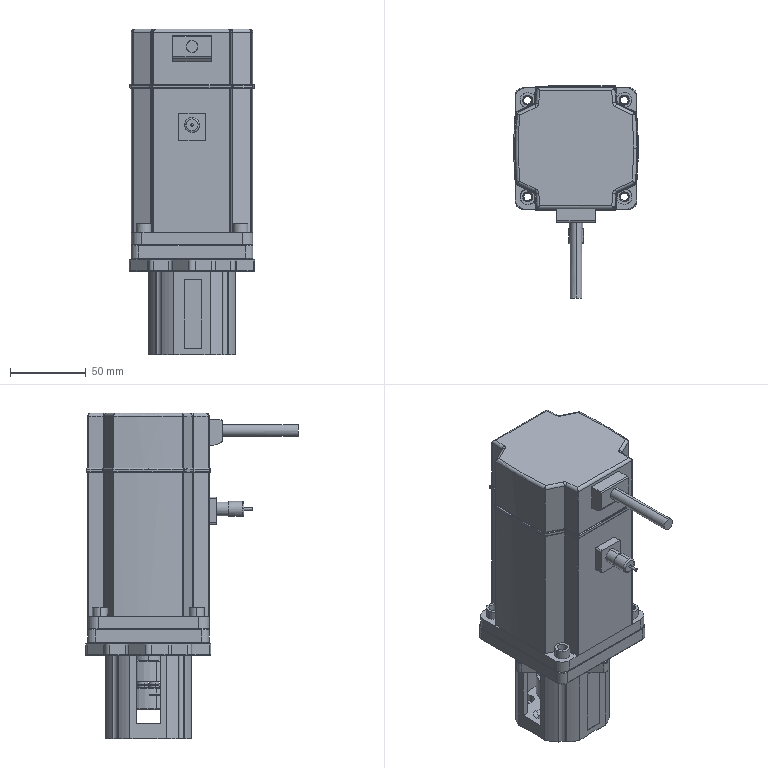Part | STEP file | Copy of 750W motor assembly (universal motor base)^K50A-1H20-S(formula driven)-L300-motor left- | 4 solids | 805 faces | box 82.368 x 139.887 x 214.5 mm | volume 943398 mm3 | cylinder 372 | plane 229 | cone 100 | torus 80 | sphere 16 | spline 8 | commonest cylinder face diameters 1 x80 7 x34 8 x23 6 x22 3.3 x21 2 x18